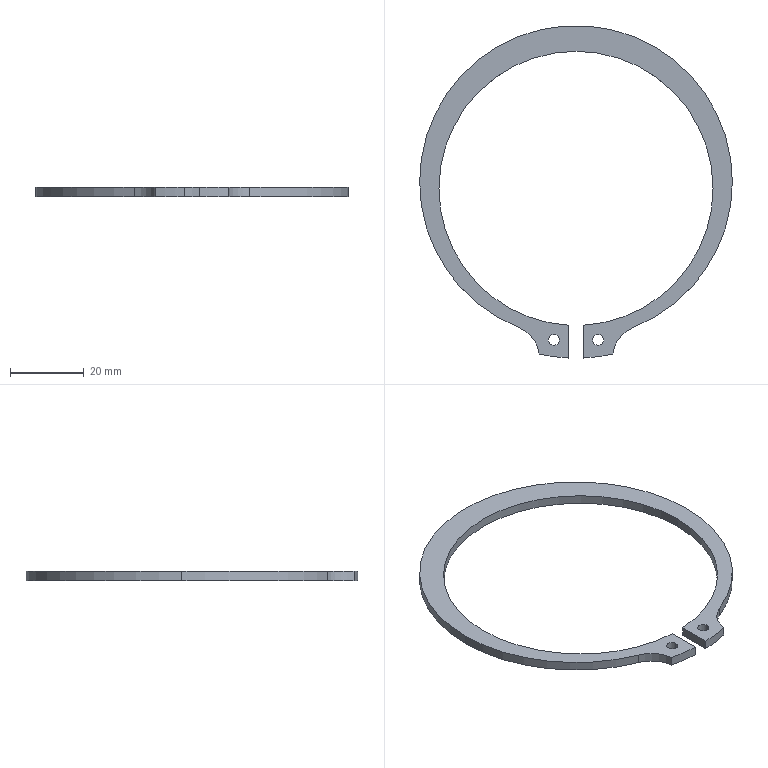Part | SolidWorks | features BaseBody 1 | 1 solid | 18 faces | box 85 x 90.347 x 2.5 mm | volume 3471 mm3 | cylinder 14 | plane 4 | commonest cylinder face diameters 3 x4 74.5 x3 85 x3 18 x2 92.28 x2
STEP:
#1=CARTESIAN_POINT('',(42.5,0.,-2.5));
#2=VERTEX_POINT('',#1);
#3=CARTESIAN_POINT('',(-42.5,0.,-2.5));
#4=VERTEX_POINT('',#3);
#5=CARTESIAN_POINT('',(0.,0.,-2.5));
#6=DIRECTION('',(0.,0.,1.));
#7=DIRECTION('',(1.,0.,0.));
#8=AXIS2_PLACEMENT_3D('',#5,#6,#7);
#9=CIRCLE('',#8,42.5);
#10=EDGE_CURVE('',#2,#4,#9,.T.);
#11=ORIENTED_EDGE('',*,*,#10,.T.);
#12=CARTESIAN_POINT('',(-42.5,0.,0.));
#13=VERTEX_POINT('',#12);
#14=CARTESIAN_POINT('',(-42.5,0.,-2.5));
#15=DIRECTION('',(0.,0.,1.));
#16=VECTOR('',#15,1000.);
#17=LINE('',#14,#16);
#18=EDGE_CURVE('',#4,#13,#17,.T.);
#19=ORIENTED_EDGE('',*,*,#18,.T.);
#20=CARTESIAN_POINT('',(42.5,0.,0.));
#21=VERTEX_POINT('',#20);
#22=CARTESIAN_POINT('',(0.,0.,0.));
#23=DIRECTION('',(0.,0.,-1.));
#24=DIRECTION('',(1.,0.,0.));
#25=AXIS2_PLACEMENT_3D('',#22,#23,#24);
#26=CIRCLE('',#25,42.5);
#27=EDGE_CURVE('',#13,#21,#26,.T.);
#28=ORIENTED_EDGE('',*,*,#27,.T.);
#29=CARTESIAN_POINT('',(42.5,0.,-2.5));
#30=DIRECTION('',(0.,0.,1.));
#31=VECTOR('',#30,1000.);
#32=LINE('',#29,#31);
#33=EDGE_CURVE('',#2,#21,#32,.T.);
#34=ORIENTED_EDGE('',*,*,#33,.F.);
#35=EDGE_LOOP('',(#11,#19,#28,#34));
#36=FACE_OUTER_BOUND('',#35,.T.);
#37=CARTESIAN_POINT('',(0.,0.,-2.5));
#38=DIRECTION('',(0.,0.,1.));
#39=DIRECTION('',(1.,0.,0.));
#40=AXIS2_PLACEMENT_3D('',#37,#38,#39);
#41=CYLINDRICAL_SURFACE('',#40,42.5);
#42=ADVANCED_FACE('',(#36),#41,.T.);
#43=CARTESIAN_POINT('',(15.624,-39.524,-2.5));
#44=VERTEX_POINT('',#43);
#45=CARTESIAN_POINT('',(0.,0.,-2.5));
#46=DIRECTION('',(0.,0.,1.));
#47=DIRECTION('',(1.,0.,0.));
#48=AXIS2_PLACEMENT_3D('',#45,#46,#47);
#49=CIRCLE('',#48,42.5);
#50=EDGE_CURVE('',#44,#2,#49,.T.);
#51=ORIENTED_EDGE('',*,*,#50,.T.);
#52=ORIENTED_EDGE('',*,*,#33,.T.);
#53=CARTESIAN_POINT('',(15.624,-39.524,0.));
#54=VERTEX_POINT('',#53);
#55=CARTESIAN_POINT('',(0.,0.,0.));
#56=DIRECTION('',(0.,0.,-1.));
#57=DIRECTION('',(1.,0.,0.));
#58=AXIS2_PLACEMENT_3D('',#55,#56,#57);
#59=CIRCLE('',#58,42.5);
#60=EDGE_CURVE('',#21,#54,#59,.T.);
#61=ORIENTED_EDGE('',*,*,#60,.T.);
#62=CARTESIAN_POINT('',(15.624,-39.524,-2.5));
#63=DIRECTION('',(0.,0.,-1.));
#64=VECTOR('',#63,1000.);
#65=LINE('',#62,#64);
#66=EDGE_CURVE('',#54,#44,#65,.T.);
#67=ORIENTED_EDGE('',*,*,#66,.T.);
#68=EDGE_LOOP('',(#51,#52,#61,#67));
#69=FACE_OUTER_BOUND('',#68,.T.);
#70=CARTESIAN_POINT('',(0.,0.,-2.5));
#71=DIRECTION('',(0.,0.,1.));
#72=DIRECTION('',(1.,0.,0.));
#73=AXIS2_PLACEMENT_3D('',#70,#71,#72);
#74=CYLINDRICAL_SURFACE('',#73,42.5);
#75=ADVANCED_FACE('',(#69),#74,.T.);
#76=CARTESIAN_POINT('',(-2.,-38.946,-2.5));
#77=VERTEX_POINT('',#76);
#78=CARTESIAN_POINT('',(-37.25,-1.75,-2.5));
#79=VERTEX_POINT('',#78);
#80=CARTESIAN_POINT('',(0.,-1.75,-2.5));
#81=DIRECTION('',(0.,0.,-1.));
#82=DIRECTION('',(1.,0.,0.));
#83=AXIS2_PLACEMENT_3D('',#80,#81,#82);
#84=CIRCLE('',#83,37.25);
#85=EDGE_CURVE('',#77,#79,#84,.T.);
#86=ORIENTED_EDGE('',*,*,#85,.T.);
#87=CARTESIAN_POINT('',(-37.25,-1.75,0.));
#88=VERTEX_POINT('',#87);
#89=CARTESIAN_POINT('',(-37.25,-1.75,-2.5));
#90=DIRECTION('',(0.,0.,1.));
#91=VECTOR('',#90,1000.);
#92=LINE('',#89,#91);
#93=EDGE_CURVE('',#79,#88,#92,.T.);
#94=ORIENTED_EDGE('',*,*,#93,.T.);
#95=CARTESIAN_POINT('',(-2.,-38.946,0.));
#96=VERTEX_POINT('',#95);
#97=CARTESIAN_POINT('',(0.,-1.75,0.));
#98=DIRECTION('',(0.,0.,-1.));
#99=DIRECTION('',(1.,0.,0.));
#100=AXIS2_PLACEMENT_3D('',#97,#98,#99);
#101=CIRCLE('',#100,37.25);
#102=EDGE_CURVE('',#96,#88,#101,.T.);
#103=ORIENTED_EDGE('',*,*,#102,.F.);
#104=CARTESIAN_POINT('',(-2.,-38.946,-2.5));
#105=DIRECTION('',(0.,0.,1.));
#106=VECTOR('',#105,1000.);
#107=LINE('',#104,#106);
#108=EDGE_CURVE('',#77,#96,#107,.T.);
#109=ORIENTED_EDGE('',*,*,#108,.F.);
#110=EDGE_LOOP('',(#86,#94,#103,#109));
#111=FACE_OUTER_BOUND('',#110,.T.);
#112=CARTESIAN_POINT('',(0.,-1.75,-2.5));
#113=DIRECTION('',(0.,0.,1.));
#114=DIRECTION('',(1.,0.,0.));
#115=AXIS2_PLACEMENT_3D('',#112,#113,#114);
#116=CYLINDRICAL_SURFACE('',#115,37.25);
#117=ADVANCED_FACE('',(#111),#116,.F.);
#118=ORIENTED_EDGE('',*,*,#93,.F.);
#119=CARTESIAN_POINT('',(37.25,-1.75,-2.5));
#120=VERTEX_POINT('',#119);
#121=CARTESIAN_POINT('',(0.,-1.75,-2.5));
#122=DIRECTION('',(0.,0.,-1.));
#123=DIRECTION('',(1.,0.,0.));
#124=AXIS2_PLACEMENT_3D('',#121,#122,#123);
#125=CIRCLE('',#124,37.25);
#126=EDGE_CURVE('',#79,#120,#125,.T.);
#127=ORIENTED_EDGE('',*,*,#126,.T.);
#128=CARTESIAN_POINT('',(37.25,-1.75,0.));
#129=VERTEX_POINT('',#128);
#130=CARTESIAN_POINT('',(37.25,-1.75,-2.5));
#131=DIRECTION('',(0.,0.,1.));
#132=VECTOR('',#131,1000.);
#133=LINE('',#130,#132);
#134=EDGE_CURVE('',#120,#129,#133,.T.);
#135=ORIENTED_EDGE('',*,*,#134,.T.);
#136=CARTESIAN_POINT('',(0.,-1.75,0.));
#137=DIRECTION('',(0.,0.,-1.));
#138=DIRECTION('',(1.,0.,0.));
#139=AXIS2_PLACEMENT_3D('',#136,#137,#138);
#140=CIRCLE('',#139,37.25);
#141=EDGE_CURVE('',#88,#129,#140,.T.);
#142=ORIENTED_EDGE('',*,*,#141,.F.);
#143=EDGE_LOOP('',(#118,#127,#135,#142));
#144=FACE_OUTER_BOUND('',#143,.T.);
#145=CARTESIAN_POINT('',(0.,-1.75,-2.5));
#146=DIRECTION('',(0.,0.,1.));
#147=DIRECTION('',(1.,0.,0.));
#148=AXIS2_PLACEMENT_3D('',#145,#146,#147);
#149=CYLINDRICAL_SURFACE('',#148,37.25);
#150=ADVANCED_FACE('',(#144),#149,.F.);
#151=CARTESIAN_POINT('',(-4.5,-42.915,-2.5));
#152=VERTEX_POINT('',#151);
#153=CARTESIAN_POINT('',(-7.5,-42.915,-2.5));
#154=VERTEX_POINT('',#153);
#155=CARTESIAN_POINT('',(-6.,-42.915,-2.5));
#156=DIRECTION('',(0.,0.,-1.));
#157=DIRECTION('',(1.,0.,0.));
#158=AXIS2_PLACEMENT_3D('',#155,#156,#157);
#159=CIRCLE('',#158,1.5);
#160=EDGE_CURVE('',#152,#154,#159,.T.);
#161=ORIENTED_EDGE('',*,*,#160,.T.);
#162=CARTESIAN_POINT('',(-7.5,-42.915,0.));
#163=VERTEX_POINT('',#162);
#164=CARTESIAN_POINT('',(-7.5,-42.915,-2.5));
#165=DIRECTION('',(0.,0.,1.));
#166=VECTOR('',#165,1000.);
#167=LINE('',#164,#166);
#168=EDGE_CURVE('',#154,#163,#167,.T.);
#169=ORIENTED_EDGE('',*,*,#168,.T.);
#170=CARTESIAN_POINT('',(-4.5,-42.915,0.));
#171=VERTEX_POINT('',#170);
#172=CARTESIAN_POINT('',(-6.,-42.915,0.));
#173=DIRECTION('',(0.,0.,-1.));
#174=DIRECTION('',(1.,0.,0.));
#175=AXIS2_PLACEMENT_3D('',#172,#173,#174);
#176=CIRCLE('',#175,1.5);
#177=EDGE_CURVE('',#171,#163,#176,.T.);
#178=ORIENTED_EDGE('',*,*,#177,.F.);
#179=CARTESIAN_POINT('',(-4.5,-42.915,-2.5));
#180=DIRECTION('',(0.,0.,1.));
#181=VECTOR('',#180,1000.);
#182=LINE('',#179,#181);
#183=EDGE_CURVE('',#152,#171,#182,.T.);
#184=ORIENTED_EDGE('',*,*,#183,.F.);
#185=EDGE_LOOP('',(#161,#169,#178,#184));
#186=FACE_OUTER_BOUND('',#185,.T.);
#187=CARTESIAN_POINT('',(-6.,-42.915,-2.5));
#188=DIRECTION('',(0.,0.,1.));
#189=DIRECTION('',(1.,0.,0.));
#190=AXIS2_PLACEMENT_3D('',#187,#188,#189);
#191=CYLINDRICAL_SURFACE('',#190,1.5);
#192=ADVANCED_FACE('',(#186),#191,.F.);
#193=CARTESIAN_POINT('',(7.5,-42.915,-2.5));
#194=VERTEX_POINT('',#193);
#195=CARTESIAN_POINT('',(4.5,-42.915,-2.5));
#196=VERTEX_POINT('',#195);
#197=CARTESIAN_POINT('',(6.,-42.915,-2.5));
#198=DIRECTION('',(0.,0.,-1.));
#199=DIRECTION('',(1.,0.,0.));
#200=AXIS2_PLACEMENT_3D('',#197,#198,#199);
#201=CIRCLE('',#200,1.5);
#202=EDGE_CURVE('',#194,#196,#201,.T.);
#203=ORIENTED_EDGE('',*,*,#202,.T.);
#204=CARTESIAN_POINT('',(4.5,-42.915,0.));
#205=VERTEX_POINT('',#204);
#206=CARTESIAN_POINT('',(4.5,-42.915,-2.5));
#207=DIRECTION('',(0.,0.,1.));
#208=VECTOR('',#207,1000.);
#209=LINE('',#206,#208);
#210=EDGE_CURVE('',#196,#205,#209,.T.);
#211=ORIENTED_EDGE('',*,*,#210,.T.);
#212=CARTESIAN_POINT('',(7.5,-42.915,0.));
#213=VERTEX_POINT('',#212);
#214=CARTESIAN_POINT('',(6.,-42.915,0.));
#215=DIRECTION('',(0.,0.,-1.));
#216=DIRECTION('',(1.,0.,0.));
#217=AXIS2_PLACEMENT_3D('',#214,#215,#216);
#218=CIRCLE('',#217,1.5);
#219=EDGE_CURVE('',#213,#205,#218,.T.);
#220=ORIENTED_EDGE('',*,*,#219,.F.);
#221=CARTESIAN_POINT('',(7.5,-42.915,-2.5));
#222=DIRECTION('',(0.,0.,1.));
#223=VECTOR('',#222,1000.);
#224=LINE('',#221,#223);
#225=EDGE_CURVE('',#194,#213,#224,.T.);
#226=ORIENTED_EDGE('',*,*,#225,.F.);
#227=EDGE_LOOP('',(#203,#211,#220,#226));
#228=FACE_OUTER_BOUND('',#227,.T.);
#229=CARTESIAN_POINT('',(6.,-42.915,-2.5));
#230=DIRECTION('',(0.,0.,1.));
#231=DIRECTION('',(1.,0.,0.));
#232=AXIS2_PLACEMENT_3D('',#229,#230,#231);
#233=CYLINDRICAL_SURFACE('',#232,1.5);
#234=ADVANCED_FACE('',(#228),#233,.F.);
#235=CARTESIAN_POINT('',(10.,-46.793,-2.5));
#236=VERTEX_POINT('',#235);
#237=CARTESIAN_POINT('',(18.932,-47.894,-2.5));
#238=DIRECTION('',(0.,0.,-1.));
#239=DIRECTION('',(-1.,0.,0.));
#240=AXIS2_PLACEMENT_3D('',#237,#238,#239);
#241=CIRCLE('',#240,9.);
#242=EDGE_CURVE('',#236,#44,#241,.T.);
#243=ORIENTED_EDGE('',*,*,#242,.F.);
#244=CARTESIAN_POINT('',(2.,-47.847,-2.5));
#245=VERTEX_POINT('',#244);
#246=CARTESIAN_POINT('',(0.,-1.75,-2.5));
#247=DIRECTION('',(0.,0.,1.));
#248=DIRECTION('',(1.,0.,0.));
#249=AXIS2_PLACEMENT_3D('',#246,#247,#248);
#250=CIRCLE('',#249,46.14);
#251=EDGE_CURVE('',#245,#236,#250,.T.);
#252=ORIENTED_EDGE('',*,*,#251,.F.);
#253=CARTESIAN_POINT('',(2.,-38.946,-2.5));
#254=VERTEX_POINT('',#253);
#255=CARTESIAN_POINT('',(2.,0.,-2.5));
#256=DIRECTION('',(0.,-1.,0.));
#257=VECTOR('',#256,1000.);
#258=LINE('',#255,#257);
#259=EDGE_CURVE('',#254,#245,#258,.T.);
#260=ORIENTED_EDGE('',*,*,#259,.F.);
#261=CARTESIAN_POINT('',(0.,-1.75,-2.5));
#262=DIRECTION('',(0.,0.,-1.));
#263=DIRECTION('',(1.,0.,0.));
#264=AXIS2_PLACEMENT_3D('',#261,#262,#263);
#265=CIRCLE('',#264,37.25);
#266=EDGE_CURVE('',#120,#254,#265,.T.);
#267=ORIENTED_EDGE('',*,*,#266,.F.);
#268=ORIENTED_EDGE('',*,*,#126,.F.);
#269=ORIENTED_EDGE('',*,*,#85,.F.);
#270=CARTESIAN_POINT('',(-2.,-47.847,-2.5));
#271=VERTEX_POINT('',#270);
#272=CARTESIAN_POINT('',(-2.,0.,-2.5));
#273=DIRECTION('',(0.,1.,0.));
#274=VECTOR('',#273,1000.);
#275=LINE('',#272,#274);
#276=EDGE_CURVE('',#271,#77,#275,.T.);
#277=ORIENTED_EDGE('',*,*,#276,.F.);
#278=CARTESIAN_POINT('',(-10.,-46.793,-2.5));
#279=VERTEX_POINT('',#278);
#280=CARTESIAN_POINT('',(0.,-1.75,-2.5));
#281=DIRECTION('',(0.,0.,1.));
#282=DIRECTION('',(1.,0.,0.));
#283=AXIS2_PLACEMENT_3D('',#280,#281,#282);
#284=CIRCLE('',#283,46.14);
#285=EDGE_CURVE('',#279,#271,#284,.T.);
#286=ORIENTED_EDGE('',*,*,#285,.F.);
#287=CARTESIAN_POINT('',(-15.624,-39.524,-2.5));
#288=VERTEX_POINT('',#287);
#289=CARTESIAN_POINT('',(-18.932,-47.894,-2.5));
#290=DIRECTION('',(0.,0.,-1.));
#291=DIRECTION('',(-1.,0.,0.));
#292=AXIS2_PLACEMENT_3D('',#289,#290,#291);
#293=CIRCLE('',#292,9.);
#294=EDGE_CURVE('',#288,#279,#293,.T.);
#295=ORIENTED_EDGE('',*,*,#294,.F.);
#296=CARTESIAN_POINT('',(0.,0.,-2.5));
#297=DIRECTION('',(0.,0.,1.));
#298=DIRECTION('',(1.,0.,0.));
#299=AXIS2_PLACEMENT_3D('',#296,#297,#298);
#300=CIRCLE('',#299,42.5);
#301=EDGE_CURVE('',#4,#288,#300,.T.);
#302=ORIENTED_EDGE('',*,*,#301,.F.);
#303=ORIENTED_EDGE('',*,*,#10,.F.);
#304=ORIENTED_EDGE('',*,*,#50,.F.);
#305=EDGE_LOOP('',(#243,#252,#260,#267,#268,#269,#277,#286,#295,#302,#303,#304));
#306=FACE_OUTER_BOUND('',#305,.T.);
#307=ORIENTED_EDGE('',*,*,#160,.F.);
#308=CARTESIAN_POINT('',(-6.,-42.915,-2.5));
#309=DIRECTION('',(0.,0.,-1.));
#310=DIRECTION('',(1.,0.,0.));
#311=AXIS2_PLACEMENT_3D('',#308,#309,#310);
#312=CIRCLE('',#311,1.5);
#313=EDGE_CURVE('',#154,#152,#312,.T.);
#314=ORIENTED_EDGE('',*,*,#313,.F.);
#315=EDGE_LOOP('',(#307,#314));
#316=FACE_BOUND('',#315,.T.);
#317=ORIENTED_EDGE('',*,*,#202,.F.);
#318=CARTESIAN_POINT('',(6.,-42.915,-2.5));
#319=DIRECTION('',(0.,0.,-1.));
#320=DIRECTION('',(1.,0.,0.));
#321=AXIS2_PLACEMENT_3D('',#318,#319,#320);
#322=CIRCLE('',#321,1.5);
#323=EDGE_CURVE('',#196,#194,#322,.T.);
#324=ORIENTED_EDGE('',*,*,#323,.F.);
#325=EDGE_LOOP('',(#317,#324));
#326=FACE_BOUND('',#325,.T.);
#327=CARTESIAN_POINT('',(0.,0.,-2.5));
#328=DIRECTION('',(0.,0.,1.));
#329=DIRECTION('',(1.,0.,0.));
#330=AXIS2_PLACEMENT_3D('',#327,#328,#329);
#331=PLANE('',#330);
#332=ADVANCED_FACE('',(#306,#316,#326),#331,.F.);
#333=ORIENTED_EDGE('',*,*,#18,.F.);
#334=ORIENTED_EDGE('',*,*,#301,.T.);
#335=CARTESIAN_POINT('',(-15.624,-39.524,0.));
#336=VERTEX_POINT('',#335);
#337=CARTESIAN_POINT('',(-15.624,-39.524,-2.5));
#338=DIRECTION('',(0.,0.,1.));
#339=VECTOR('',#338,1000.);
#340=LINE('',#337,#339);
#341=EDGE_CURVE('',#288,#336,#340,.T.);
#342=ORIENTED_EDGE('',*,*,#341,.T.);
#343=CARTESIAN_POINT('',(0.,0.,0.));
#344=DIRECTION('',(0.,0.,-1.));
#345=DIRECTION('',(1.,0.,0.));
#346=AXIS2_PLACEMENT_3D('',#343,#344,#345);
#347=CIRCLE('',#346,42.5);
#348=EDGE_CURVE('',#336,#13,#347,.T.);
#349=ORIENTED_EDGE('',*,*,#348,.T.);
#350=EDGE_LOOP('',(#333,#334,#342,#349));
#351=FACE_OUTER_BOUND('',#350,.T.);
#352=CARTESIAN_POINT('',(0.,0.,-2.5));
#353=DIRECTION('',(0.,0.,1.));
#354=DIRECTION('',(1.,0.,0.));
#355=AXIS2_PLACEMENT_3D('',#352,#353,#354);
#356=CYLINDRICAL_SURFACE('',#355,42.5);
#357=ADVANCED_FACE('',(#351),#356,.T.);
#358=ORIENTED_EDGE('',*,*,#66,.F.);
#359=CARTESIAN_POINT('',(10.,-46.793,0.));
#360=VERTEX_POINT('',#359);
#361=CARTESIAN_POINT('',(18.932,-47.894,0.));
#362=DIRECTION('',(0.,0.,-1.));
#363=DIRECTION('',(-1.,0.,0.));
#364=AXIS2_PLACEMENT_3D('',#361,#362,#363);
#365=CIRCLE('',#364,9.);
#366=EDGE_CURVE('',#360,#54,#365,.T.);
#367=ORIENTED_EDGE('',*,*,#366,.F.);
#368=CARTESIAN_POINT('',(10.,-46.793,-2.5));
#369=DIRECTION('',(0.,0.,1.));
#370=VECTOR('',#369,1000.);
#371=LINE('',#368,#370);
#372=EDGE_CURVE('',#236,#360,#371,.T.);
#373=ORIENTED_EDGE('',*,*,#372,.F.);
#374=ORIENTED_EDGE('',*,*,#242,.T.);
#375=EDGE_LOOP('',(#358,#367,#373,#374));
#376=FACE_OUTER_BOUND('',#375,.T.);
#377=CARTESIAN_POINT('',(18.932,-47.894,-2.5));
#378=DIRECTION('',(0.,0.,-1.));
#379=DIRECTION('',(-1.,0.,0.));
#380=AXIS2_PLACEMENT_3D('',#377,#378,#379);
#381=CYLINDRICAL_SURFACE('',#380,9.);
#382=ADVANCED_FACE('',(#376),#381,.F.);
#383=ORIENTED_EDGE('',*,*,#251,.T.);
#384=ORIENTED_EDGE('',*,*,#372,.T.);
#385=CARTESIAN_POINT('',(2.,-47.847,0.));
#386=VERTEX_POINT('',#385);
#387=CARTESIAN_POINT('',(0.,-1.75,0.));
#388=DIRECTION('',(0.,0.,-1.));
#389=DIRECTION('',(1.,0.,0.));
#390=AXIS2_PLACEMENT_3D('',#387,#388,#389);
#391=CIRCLE('',#390,46.14);
#392=EDGE_CURVE('',#360,#386,#391,.T.);
#393=ORIENTED_EDGE('',*,*,#392,.T.);
#394=CARTESIAN_POINT('',(2.,-47.847,-2.5));
#395=DIRECTION('',(0.,0.,-1.));
#396=VECTOR('',#395,1000.);
#397=LINE('',#394,#396);
#398=EDGE_CURVE('',#386,#245,#397,.T.);
#399=ORIENTED_EDGE('',*,*,#398,.T.);
#400=EDGE_LOOP('',(#383,#384,#393,#399));
#401=FACE_OUTER_BOUND('',#400,.T.);
#402=CARTESIAN_POINT('',(0.,-1.75,-2.5));
#403=DIRECTION('',(0.,0.,1.));
#404=DIRECTION('',(1.,0.,0.));
#405=AXIS2_PLACEMENT_3D('',#402,#403,#404);
#406=CYLINDRICAL_SURFACE('',#405,46.14);
#407=ADVANCED_FACE('',(#401),#406,.T.);
#408=ORIENTED_EDGE('',*,*,#259,.T.);
#409=ORIENTED_EDGE('',*,*,#398,.F.);
#410=CARTESIAN_POINT('',(2.,-38.946,0.));
#411=VERTEX_POINT('',#410);
#412=CARTESIAN_POINT('',(2.,-47.847,0.));
#413=DIRECTION('',(0.,1.,0.));
#414=VECTOR('',#413,1000.);
#415=LINE('',#412,#414);
#416=EDGE_CURVE('',#386,#411,#415,.T.);
#417=ORIENTED_EDGE('',*,*,#416,.T.);
#418=CARTESIAN_POINT('',(2.,-38.946,-2.5));
#419=DIRECTION('',(0.,0.,-1.));
#420=VECTOR('',#419,1000.);
#421=LINE('',#418,#420);
#422=EDGE_CURVE('',#411,#254,#421,.T.);
#423=ORIENTED_EDGE('',*,*,#422,.T.);
#424=EDGE_LOOP('',(#408,#409,#417,#423));
#425=FACE_OUTER_BOUND('',#424,.T.);
#426=CARTESIAN_POINT('',(2.,-47.847,-2.5));
#427=DIRECTION('',(-1.,0.,0.));
#428=DIRECTION('',(0.,-1.,0.));
#429=AXIS2_PLACEMENT_3D('',#426,#427,#428);
#430=PLANE('',#429);
#431=ADVANCED_FACE('',(#425),#430,.T.);
#432=ORIENTED_EDGE('',*,*,#134,.F.);
#433=ORIENTED_EDGE('',*,*,#266,.T.);
#434=ORIENTED_EDGE('',*,*,#422,.F.);
#435=CARTESIAN_POINT('',(0.,-1.75,0.));
#436=DIRECTION('',(0.,0.,-1.));
#437=DIRECTION('',(1.,0.,0.));
#438=AXIS2_PLACEMENT_3D('',#435,#436,#437);
#439=CIRCLE('',#438,37.25);
#440=EDGE_CURVE('',#129,#411,#439,.T.);
#441=ORIENTED_EDGE('',*,*,#440,.F.);
#442=EDGE_LOOP('',(#432,#433,#434,#441));
#443=FACE_OUTER_BOUND('',#442,.T.);
#444=CARTESIAN_POINT('',(0.,-1.75,-2.5));
#445=DIRECTION('',(0.,0.,1.));
#446=DIRECTION('',(1.,0.,0.));
#447=AXIS2_PLACEMENT_3D('',#444,#445,#446);
#448=CYLINDRICAL_SURFACE('',#447,37.25);
#449=ADVANCED_FACE('',(#443),#448,.F.);
#450=ORIENTED_EDGE('',*,*,#276,.T.);
#451=ORIENTED_EDGE('',*,*,#108,.T.);
#452=CARTESIAN_POINT('',(-2.,-47.847,0.));
#453=VERTEX_POINT('',#452);
#454=CARTESIAN_POINT('',(-2.,-47.847,0.));
#455=DIRECTION('',(0.,-1.,0.));
#456=VECTOR('',#455,1000.);
#457=LINE('',#454,#456);
#458=EDGE_CURVE('',#96,#453,#457,.T.);
#459=ORIENTED_EDGE('',*,*,#458,.T.);
#460=CARTESIAN_POINT('',(-2.,-47.847,-2.5));
#461=DIRECTION('',(0.,0.,-1.));
#462=VECTOR('',#461,1000.);
#463=LINE('',#460,#462);
#464=EDGE_CURVE('',#453,#271,#463,.T.);
#465=ORIENTED_EDGE('',*,*,#464,.T.);
#466=EDGE_LOOP('',(#450,#451,#459,#465));
#467=FACE_OUTER_BOUND('',#466,.T.);
#468=CARTESIAN_POINT('',(-2.,-47.847,-2.5));
#469=DIRECTION('',(1.,0.,0.));
#470=DIRECTION('',(0.,0.,-1.));
#471=AXIS2_PLACEMENT_3D('',#468,#469,#470);
#472=PLANE('',#471);
#473=ADVANCED_FACE('',(#467),#472,.T.);
#474=ORIENTED_EDGE('',*,*,#285,.T.);
#475=ORIENTED_EDGE('',*,*,#464,.F.);
#476=CARTESIAN_POINT('',(-10.,-46.793,0.));
#477=VERTEX_POINT('',#476);
#478=CARTESIAN_POINT('',(0.,-1.75,0.));
#479=DIRECTION('',(0.,0.,-1.));
#480=DIRECTION('',(1.,0.,0.));
#481=AXIS2_PLACEMENT_3D('',#478,#479,#480);
#482=CIRCLE('',#481,46.14);
#483=EDGE_CURVE('',#453,#477,#482,.T.);
#484=ORIENTED_EDGE('',*,*,#483,.T.);
#485=CARTESIAN_POINT('',(-10.,-46.793,-2.5));
#486=DIRECTION('',(0.,0.,-1.));
#487=VECTOR('',#486,1000.);
#488=LINE('',#485,#487);
#489=EDGE_CURVE('',#477,#279,#488,.T.);
#490=ORIENTED_EDGE('',*,*,#489,.T.);
#491=EDGE_LOOP('',(#474,#475,#484,#490));
#492=FACE_OUTER_BOUND('',#491,.T.);
#493=CARTESIAN_POINT('',(0.,-1.75,-2.5));
#494=DIRECTION('',(0.,0.,1.));
#495=DIRECTION('',(1.,0.,0.));
#496=AXIS2_PLACEMENT_3D('',#493,#494,#495);
#497=CYLINDRICAL_SURFACE('',#496,46.14);
#498=ADVANCED_FACE('',(#492),#497,.T.);
#499=ORIENTED_EDGE('',*,*,#489,.F.);
#500=CARTESIAN_POINT('',(-18.932,-47.894,0.));
#501=DIRECTION('',(0.,0.,-1.));
#502=DIRECTION('',(-1.,0.,0.));
#503=AXIS2_PLACEMENT_3D('',#500,#501,#502);
#504=CIRCLE('',#503,9.);
#505=EDGE_CURVE('',#336,#477,#504,.T.);
#506=ORIENTED_EDGE('',*,*,#505,.F.);
#507=ORIENTED_EDGE('',*,*,#341,.F.);
#508=ORIENTED_EDGE('',*,*,#294,.T.);
#509=EDGE_LOOP('',(#499,#506,#507,#508));
#510=FACE_OUTER_BOUND('',#509,.T.);
#511=CARTESIAN_POINT('',(-18.932,-47.894,-2.5));
#512=DIRECTION('',(0.,0.,-1.));
#513=DIRECTION('',(-1.,0.,0.));
#514=AXIS2_PLACEMENT_3D('',#511,#512,#513);
#515=CYLINDRICAL_SURFACE('',#514,9.);
#516=ADVANCED_FACE('',(#510),#515,.F.);
#517=ORIENTED_EDGE('',*,*,#168,.F.);
#518=ORIENTED_EDGE('',*,*,#313,.T.);
#519=ORIENTED_EDGE('',*,*,#183,.T.);
#520=CARTESIAN_POINT('',(-6.,-42.915,0.));
#521=DIRECTION('',(0.,0.,-1.));
#522=DIRECTION('',(1.,0.,0.));
#523=AXIS2_PLACEMENT_3D('',#520,#521,#522);
#524=CIRCLE('',#523,1.5);
#525=EDGE_CURVE('',#163,#171,#524,.T.);
#526=ORIENTED_EDGE('',*,*,#525,.F.);
#527=EDGE_LOOP('',(#517,#518,#519,#526));
#528=FACE_OUTER_BOUND('',#527,.T.);
#529=CARTESIAN_POINT('',(-6.,-42.915,-2.5));
#530=DIRECTION('',(0.,0.,1.));
#531=DIRECTION('',(1.,0.,0.));
#532=AXIS2_PLACEMENT_3D('',#529,#530,#531);
#533=CYLINDRICAL_SURFACE('',#532,1.5);
#534=ADVANCED_FACE('',(#528),#533,.F.);
#535=ORIENTED_EDGE('',*,*,#210,.F.);
#536=ORIENTED_EDGE('',*,*,#323,.T.);
#537=ORIENTED_EDGE('',*,*,#225,.T.);
#538=CARTESIAN_POINT('',(6.,-42.915,0.));
#539=DIRECTION('',(0.,0.,-1.));
#540=DIRECTION('',(1.,0.,0.));
#541=AXIS2_PLACEMENT_3D('',#538,#539,#540);
#542=CIRCLE('',#541,1.5);
#543=EDGE_CURVE('',#205,#213,#542,.T.);
#544=ORIENTED_EDGE('',*,*,#543,.F.);
#545=EDGE_LOOP('',(#535,#536,#537,#544));
#546=FACE_OUTER_BOUND('',#545,.T.);
#547=CARTESIAN_POINT('',(6.,-42.915,-2.5));
#548=DIRECTION('',(0.,0.,1.));
#549=DIRECTION('',(1.,0.,0.));
#550=AXIS2_PLACEMENT_3D('',#547,#548,#549);
#551=CYLINDRICAL_SURFACE('',#550,1.5);
#552=ADVANCED_FACE('',(#546),#551,.F.);
#553=ORIENTED_EDGE('',*,*,#102,.T.);
#554=ORIENTED_EDGE('',*,*,#141,.T.);
#555=ORIENTED_EDGE('',*,*,#440,.T.);
#556=ORIENTED_EDGE('',*,*,#416,.F.);
#557=ORIENTED_EDGE('',*,*,#392,.F.);
#558=ORIENTED_EDGE('',*,*,#366,.T.);
#559=ORIENTED_EDGE('',*,*,#60,.F.);
#560=ORIENTED_EDGE('',*,*,#27,.F.);
#561=ORIENTED_EDGE('',*,*,#348,.F.);
#562=ORIENTED_EDGE('',*,*,#505,.T.);
#563=ORIENTED_EDGE('',*,*,#483,.F.);
#564=ORIENTED_EDGE('',*,*,#458,.F.);
#565=EDGE_LOOP('',(#553,#554,#555,#556,#557,#558,#559,#560,#561,#562,#563,#564));
#566=FACE_OUTER_BOUND('',#565,.T.);
#567=ORIENTED_EDGE('',*,*,#177,.T.);
#568=ORIENTED_EDGE('',*,*,#525,.T.);
#569=EDGE_LOOP('',(#567,#568));
#570=FACE_BOUND('',#569,.T.);
#571=ORIENTED_EDGE('',*,*,#219,.T.);
#572=ORIENTED_EDGE('',*,*,#543,.T.);
#573=EDGE_LOOP('',(#571,#572));
#574=FACE_BOUND('',#573,.T.);
#575=CARTESIAN_POINT('',(0.,0.,0.));
#576=DIRECTION('',(0.,0.,1.));
#577=DIRECTION('',(1.,0.,0.));
#578=AXIS2_PLACEMENT_3D('',#575,#576,#577);
#579=PLANE('',#578);
#580=ADVANCED_FACE('',(#566,#570,#574),#579,.T.);
#581=CLOSED_SHELL('',(#42,#75,#117,#150,#192,#234,#332,#357,#382,#407,#431,#449,#473,#498,#516,#534,#552,#580));
#582=MANIFOLD_SOLID_BREP('',#581);
#583=CARTESIAN_POINT('',(0.,0.,0.));
#584=DIRECTION('',(0.,0.,1.));
#585=DIRECTION('',(1.,0.,0.));
#586=AXIS2_PLACEMENT_3D('',#583,#584,#585);
#587=(LENGTH_UNIT()NAMED_UNIT(*)SI_UNIT(.MILLI.,.METRE.));
#588=UNCERTAINTY_MEASURE_WITH_UNIT(LENGTH_MEASURE(0.00001),#587,'','');
#589=(NAMED_UNIT(*)PLANE_ANGLE_UNIT()SI_UNIT($,.RADIAN.));
#590=(NAMED_UNIT(*)SI_UNIT($,.STERADIAN.)SOLID_ANGLE_UNIT());
#591=(GEOMETRIC_REPRESENTATION_CONTEXT(3)GLOBAL_UNCERTAINTY_ASSIGNED_CONTEXT((#588))GLOBAL_UNIT_ASSIGNED_CONTEXT((#587,#589,#590))REPRESENTATION_CONTEXT('',''));
#592=ADVANCED_BREP_SHAPE_REPRESENTATION('',(#582,#586),#591);